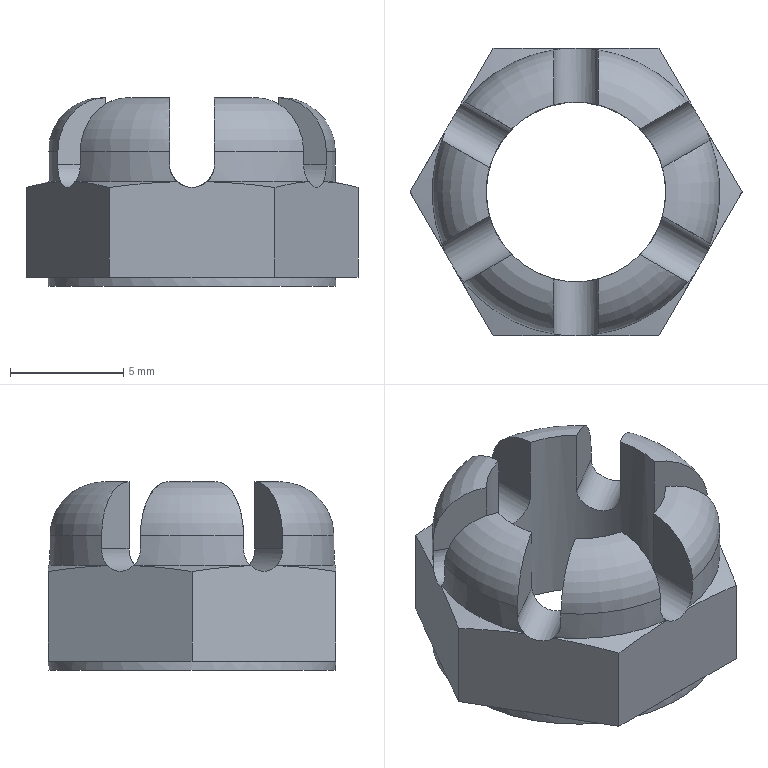Part | NX | features solid 2 | 1 solid | 51 faces | box 14.665 x 12.7 x 8.334 mm | volume 560.017 mm3 | plane 25 | cylinder 14 | torus 6 | cone 6 | commonest cylinder face diameters 12.7 x7 1.984 x6 7.938 x1